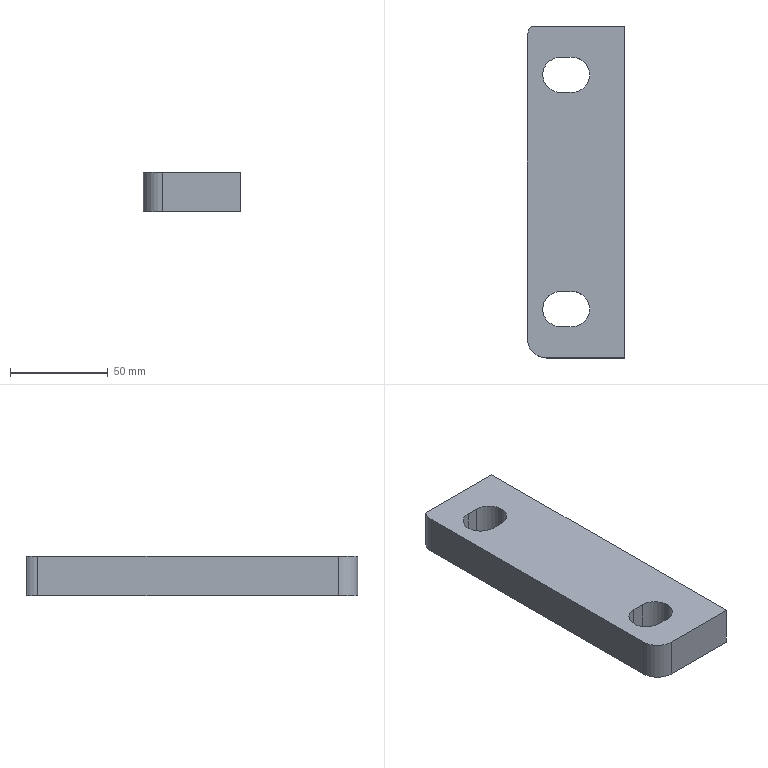Part | SolidWorks | features BaseBody 1 | 1 solid | 18 faces | box 50 x 170 x 20 mm | volume 154996 mm3 | plane 10 | cylinder 8 | commonest cylinder face diameters 18 x6 20 x2
STEP:
#1=CARTESIAN_POINT('',(-40.5,-55.,-12.5));
#2=VERTEX_POINT('',#1);
#3=CARTESIAN_POINT('',(-49.5,-46.,-12.5));
#4=VERTEX_POINT('',#3);
#5=CARTESIAN_POINT('',(-49.5,-55.,-12.5));
#6=DIRECTION('',(0.,0.,1.));
#7=DIRECTION('',(1.,0.,0.));
#8=AXIS2_PLACEMENT_3D('',#5,#6,#7);
#9=CIRCLE('',#8,9.);
#10=EDGE_CURVE('',#2,#4,#9,.T.);
#11=ORIENTED_EDGE('',*,*,#10,.F.);
#12=CARTESIAN_POINT('',(-40.5,-55.,7.5));
#13=VERTEX_POINT('',#12);
#14=CARTESIAN_POINT('',(-40.5,-55.,-12.5));
#15=DIRECTION('',(0.,0.,1.));
#16=VECTOR('',#15,1000.);
#17=LINE('',#14,#16);
#18=EDGE_CURVE('',#2,#13,#17,.T.);
#19=ORIENTED_EDGE('',*,*,#18,.T.);
#20=CARTESIAN_POINT('',(-49.5,-46.,7.5));
#21=VERTEX_POINT('',#20);
#22=CARTESIAN_POINT('',(-49.5,-55.,7.5));
#23=DIRECTION('',(0.,0.,1.));
#24=DIRECTION('',(1.,0.,0.));
#25=AXIS2_PLACEMENT_3D('',#22,#23,#24);
#26=CIRCLE('',#25,9.);
#27=EDGE_CURVE('',#13,#21,#26,.T.);
#28=ORIENTED_EDGE('',*,*,#27,.T.);
#29=CARTESIAN_POINT('',(-49.5,-46.,-12.5));
#30=DIRECTION('',(0.,0.,1.));
#31=VECTOR('',#30,1000.);
#32=LINE('',#29,#31);
#33=EDGE_CURVE('',#4,#21,#32,.T.);
#34=ORIENTED_EDGE('',*,*,#33,.F.);
#35=EDGE_LOOP('',(#11,#19,#28,#34));
#36=FACE_OUTER_BOUND('',#35,.T.);
#37=CARTESIAN_POINT('',(-49.5,-55.,-12.5));
#38=DIRECTION('',(0.,0.,1.));
#39=DIRECTION('',(1.,0.,0.));
#40=AXIS2_PLACEMENT_3D('',#37,#38,#39);
#41=CYLINDRICAL_SURFACE('',#40,9.);
#42=ADVANCED_FACE('',(#36),#41,.F.);
#43=CARTESIAN_POINT('',(-40.5,65.,-12.5));
#44=VERTEX_POINT('',#43);
#45=CARTESIAN_POINT('',(-49.5,74.,-12.5));
#46=VERTEX_POINT('',#45);
#47=CARTESIAN_POINT('',(-49.5,65.,-12.5));
#48=DIRECTION('',(0.,0.,1.));
#49=DIRECTION('',(1.,0.,0.));
#50=AXIS2_PLACEMENT_3D('',#47,#48,#49);
#51=CIRCLE('',#50,9.);
#52=EDGE_CURVE('',#44,#46,#51,.T.);
#53=ORIENTED_EDGE('',*,*,#52,.F.);
#54=CARTESIAN_POINT('',(-40.5,65.,7.5));
#55=VERTEX_POINT('',#54);
#56=CARTESIAN_POINT('',(-40.5,65.,-12.5));
#57=DIRECTION('',(0.,0.,1.));
#58=VECTOR('',#57,1000.);
#59=LINE('',#56,#58);
#60=EDGE_CURVE('',#44,#55,#59,.T.);
#61=ORIENTED_EDGE('',*,*,#60,.T.);
#62=CARTESIAN_POINT('',(-49.5,74.,7.5));
#63=VERTEX_POINT('',#62);
#64=CARTESIAN_POINT('',(-49.5,65.,7.5));
#65=DIRECTION('',(0.,0.,1.));
#66=DIRECTION('',(1.,0.,0.));
#67=AXIS2_PLACEMENT_3D('',#64,#65,#66);
#68=CIRCLE('',#67,9.);
#69=EDGE_CURVE('',#55,#63,#68,.T.);
#70=ORIENTED_EDGE('',*,*,#69,.T.);
#71=CARTESIAN_POINT('',(-49.5,74.,-12.5));
#72=DIRECTION('',(0.,0.,1.));
#73=VECTOR('',#72,1000.);
#74=LINE('',#71,#73);
#75=EDGE_CURVE('',#46,#63,#74,.T.);
#76=ORIENTED_EDGE('',*,*,#75,.F.);
#77=EDGE_LOOP('',(#53,#61,#70,#76));
#78=FACE_OUTER_BOUND('',#77,.T.);
#79=CARTESIAN_POINT('',(-49.5,65.,-12.5));
#80=DIRECTION('',(0.,0.,1.));
#81=DIRECTION('',(1.,0.,0.));
#82=AXIS2_PLACEMENT_3D('',#79,#80,#81);
#83=CYLINDRICAL_SURFACE('',#82,9.);
#84=ADVANCED_FACE('',(#78),#83,.F.);
#85=CARTESIAN_POINT('',(-22.5,-80.,7.5));
#86=VERTEX_POINT('',#85);
#87=CARTESIAN_POINT('',(-22.5,90.,7.5));
#88=VERTEX_POINT('',#87);
#89=CARTESIAN_POINT('',(-22.5,94.,7.5));
#90=DIRECTION('',(0.,1.,0.));
#91=VECTOR('',#90,1000.);
#92=LINE('',#89,#91);
#93=EDGE_CURVE('',#86,#88,#92,.T.);
#94=ORIENTED_EDGE('',*,*,#93,.F.);
#95=CARTESIAN_POINT('',(-22.5,-80.,-12.5));
#96=VERTEX_POINT('',#95);
#97=CARTESIAN_POINT('',(-22.5,-80.,12.5));
#98=DIRECTION('',(0.,0.,-1.));
#99=VECTOR('',#98,1000.);
#100=LINE('',#97,#99);
#101=EDGE_CURVE('',#86,#96,#100,.T.);
#102=ORIENTED_EDGE('',*,*,#101,.T.);
#103=CARTESIAN_POINT('',(-22.5,90.,-12.5));
#104=VERTEX_POINT('',#103);
#105=CARTESIAN_POINT('',(-22.5,94.,-12.5));
#106=DIRECTION('',(0.,1.,0.));
#107=VECTOR('',#106,1000.);
#108=LINE('',#105,#107);
#109=EDGE_CURVE('',#96,#104,#108,.T.);
#110=ORIENTED_EDGE('',*,*,#109,.T.);
#111=CARTESIAN_POINT('',(-22.5,90.,12.5));
#112=DIRECTION('',(0.,0.,-1.));
#113=VECTOR('',#112,1000.);
#114=LINE('',#111,#113);
#115=EDGE_CURVE('',#88,#104,#114,.T.);
#116=ORIENTED_EDGE('',*,*,#115,.F.);
#117=EDGE_LOOP('',(#94,#102,#110,#116));
#118=FACE_OUTER_BOUND('',#117,.T.);
#119=CARTESIAN_POINT('',(-22.5,94.,12.5));
#120=DIRECTION('',(-1.,0.,0.));
#121=DIRECTION('',(0.,-1.,0.));
#122=AXIS2_PLACEMENT_3D('',#119,#120,#121);
#123=PLANE('',#122);
#124=ADVANCED_FACE('',(#118),#123,.F.);
#125=CARTESIAN_POINT('',(-70.5,90.,7.5));
#126=VERTEX_POINT('',#125);
#127=CARTESIAN_POINT('',(-72.5,84.,7.5));
#128=VERTEX_POINT('',#127);
#129=CARTESIAN_POINT('',(-62.5,84.,7.5));
#130=DIRECTION('',(0.,0.,1.));
#131=DIRECTION('',(0.,-1.,0.));
#132=AXIS2_PLACEMENT_3D('',#129,#130,#131);
#133=CIRCLE('',#132,10.);
#134=EDGE_CURVE('',#126,#128,#133,.T.);
#135=ORIENTED_EDGE('',*,*,#134,.F.);
#136=CARTESIAN_POINT('',(-70.5,90.,-12.5));
#137=VERTEX_POINT('',#136);
#138=CARTESIAN_POINT('',(-70.5,90.,12.5));
#139=DIRECTION('',(0.,0.,1.));
#140=VECTOR('',#139,1000.);
#141=LINE('',#138,#140);
#142=EDGE_CURVE('',#137,#126,#141,.T.);
#143=ORIENTED_EDGE('',*,*,#142,.F.);
#144=CARTESIAN_POINT('',(-72.5,84.,-12.5));
#145=VERTEX_POINT('',#144);
#146=CARTESIAN_POINT('',(-62.5,84.,-12.5));
#147=DIRECTION('',(0.,0.,1.));
#148=DIRECTION('',(1.,0.,0.));
#149=AXIS2_PLACEMENT_3D('',#146,#147,#148);
#150=CIRCLE('',#149,10.);
#151=EDGE_CURVE('',#137,#145,#150,.T.);
#152=ORIENTED_EDGE('',*,*,#151,.T.);
#153=CARTESIAN_POINT('',(-72.5,84.,12.5));
#154=DIRECTION('',(0.,0.,-1.));
#155=VECTOR('',#154,1000.);
#156=LINE('',#153,#155);
#157=EDGE_CURVE('',#128,#145,#156,.T.);
#158=ORIENTED_EDGE('',*,*,#157,.F.);
#159=EDGE_LOOP('',(#135,#143,#152,#158));
#160=FACE_OUTER_BOUND('',#159,.T.);
#161=CARTESIAN_POINT('',(-62.5,84.,12.5));
#162=DIRECTION('',(0.,0.,-1.));
#163=DIRECTION('',(-1.,0.,0.));
#164=AXIS2_PLACEMENT_3D('',#161,#162,#163);
#165=CYLINDRICAL_SURFACE('',#164,10.);
#166=ADVANCED_FACE('',(#160),#165,.T.);
#167=CARTESIAN_POINT('',(-72.5,-70.,7.5));
#168=VERTEX_POINT('',#167);
#169=CARTESIAN_POINT('',(-72.5,84.,7.5));
#170=DIRECTION('',(0.,-1.,0.));
#171=VECTOR('',#170,1000.);
#172=LINE('',#169,#171);
#173=EDGE_CURVE('',#128,#168,#172,.T.);
#174=ORIENTED_EDGE('',*,*,#173,.F.);
#175=ORIENTED_EDGE('',*,*,#157,.T.);
#176=CARTESIAN_POINT('',(-72.5,-70.,-12.5));
#177=VERTEX_POINT('',#176);
#178=CARTESIAN_POINT('',(-72.5,84.,-12.5));
#179=DIRECTION('',(0.,-1.,0.));
#180=VECTOR('',#179,1000.);
#181=LINE('',#178,#180);
#182=EDGE_CURVE('',#145,#177,#181,.T.);
#183=ORIENTED_EDGE('',*,*,#182,.T.);
#184=CARTESIAN_POINT('',(-72.5,-70.,12.5));
#185=DIRECTION('',(0.,0.,-1.));
#186=VECTOR('',#185,1000.);
#187=LINE('',#184,#186);
#188=EDGE_CURVE('',#168,#177,#187,.T.);
#189=ORIENTED_EDGE('',*,*,#188,.F.);
#190=EDGE_LOOP('',(#174,#175,#183,#189));
#191=FACE_OUTER_BOUND('',#190,.T.);
#192=CARTESIAN_POINT('',(-72.5,84.,12.5));
#193=DIRECTION('',(1.,0.,0.));
#194=DIRECTION('',(0.,1.,0.));
#195=AXIS2_PLACEMENT_3D('',#192,#193,#194);
#196=PLANE('',#195);
#197=ADVANCED_FACE('',(#191),#196,.F.);
#198=CARTESIAN_POINT('',(-62.5,-80.,7.5));
#199=VERTEX_POINT('',#198);
#200=CARTESIAN_POINT('',(-62.5,-70.,7.5));
#201=DIRECTION('',(0.,0.,1.));
#202=DIRECTION('',(0.,-1.,0.));
#203=AXIS2_PLACEMENT_3D('',#200,#201,#202);
#204=CIRCLE('',#203,10.);
#205=EDGE_CURVE('',#168,#199,#204,.T.);
#206=ORIENTED_EDGE('',*,*,#205,.F.);
#207=ORIENTED_EDGE('',*,*,#188,.T.);
#208=CARTESIAN_POINT('',(-62.5,-80.,-12.5));
#209=VERTEX_POINT('',#208);
#210=CARTESIAN_POINT('',(-62.5,-70.,-12.5));
#211=DIRECTION('',(0.,0.,1.));
#212=DIRECTION('',(1.,0.,0.));
#213=AXIS2_PLACEMENT_3D('',#210,#211,#212);
#214=CIRCLE('',#213,10.);
#215=EDGE_CURVE('',#177,#209,#214,.T.);
#216=ORIENTED_EDGE('',*,*,#215,.T.);
#217=CARTESIAN_POINT('',(-62.5,-80.,12.5));
#218=DIRECTION('',(0.,0.,-1.));
#219=VECTOR('',#218,1000.);
#220=LINE('',#217,#219);
#221=EDGE_CURVE('',#199,#209,#220,.T.);
#222=ORIENTED_EDGE('',*,*,#221,.F.);
#223=EDGE_LOOP('',(#206,#207,#216,#222));
#224=FACE_OUTER_BOUND('',#223,.T.);
#225=CARTESIAN_POINT('',(-62.5,-70.,12.5));
#226=DIRECTION('',(0.,0.,-1.));
#227=DIRECTION('',(-1.,0.,0.));
#228=AXIS2_PLACEMENT_3D('',#225,#226,#227);
#229=CYLINDRICAL_SURFACE('',#228,10.);
#230=ADVANCED_FACE('',(#224),#229,.T.);
#231=CARTESIAN_POINT('',(-1372.5,-80.,7.5));
#232=DIRECTION('',(1.,0.,0.));
#233=VECTOR('',#232,1000.);
#234=LINE('',#231,#233);
#235=EDGE_CURVE('',#199,#86,#234,.T.);
#236=ORIENTED_EDGE('',*,*,#235,.F.);
#237=ORIENTED_EDGE('',*,*,#221,.T.);
#238=CARTESIAN_POINT('',(-62.5,-80.,-12.5));
#239=DIRECTION('',(1.,0.,0.));
#240=VECTOR('',#239,1000.);
#241=LINE('',#238,#240);
#242=EDGE_CURVE('',#209,#96,#241,.T.);
#243=ORIENTED_EDGE('',*,*,#242,.T.);
#244=ORIENTED_EDGE('',*,*,#101,.F.);
#245=EDGE_LOOP('',(#236,#237,#243,#244));
#246=FACE_OUTER_BOUND('',#245,.T.);
#247=CARTESIAN_POINT('',(-62.5,-80.,12.5));
#248=DIRECTION('',(0.,1.,0.));
#249=DIRECTION('',(0.,0.,1.));
#250=AXIS2_PLACEMENT_3D('',#247,#248,#249);
#251=PLANE('',#250);
#252=ADVANCED_FACE('',(#246),#251,.F.);
#253=ORIENTED_EDGE('',*,*,#142,.T.);
#254=CARTESIAN_POINT('',(-657.5,90.,7.5));
#255=DIRECTION('',(1.,0.,0.));
#256=VECTOR('',#255,1000.);
#257=LINE('',#254,#256);
#258=EDGE_CURVE('',#126,#88,#257,.T.);
#259=ORIENTED_EDGE('',*,*,#258,.T.);
#260=ORIENTED_EDGE('',*,*,#115,.T.);
#261=CARTESIAN_POINT('',(-62.5,90.,-12.5));
#262=DIRECTION('',(-1.,0.,0.));
#263=VECTOR('',#262,1000.);
#264=LINE('',#261,#263);
#265=EDGE_CURVE('',#104,#137,#264,.T.);
#266=ORIENTED_EDGE('',*,*,#265,.T.);
#267=EDGE_LOOP('',(#253,#259,#260,#266));
#268=FACE_OUTER_BOUND('',#267,.T.);
#269=CARTESIAN_POINT('',(-657.5,90.,-755.));
#270=DIRECTION('',(0.,1.,0.));
#271=DIRECTION('',(0.,0.,1.));
#272=AXIS2_PLACEMENT_3D('',#269,#270,#271);
#273=PLANE('',#272);
#274=ADVANCED_FACE('',(#268),#273,.T.);
#275=CARTESIAN_POINT('',(-55.5,-46.,-12.5));
#276=VERTEX_POINT('',#275);
#277=CARTESIAN_POINT('',(-55.5,-46.,-12.5));
#278=DIRECTION('',(-1.,0.,0.));
#279=VECTOR('',#278,1000.);
#280=LINE('',#277,#279);
#281=EDGE_CURVE('',#4,#276,#280,.T.);
#282=ORIENTED_EDGE('',*,*,#281,.T.);
#283=CARTESIAN_POINT('',(-55.5,-64.,-12.5));
#284=VERTEX_POINT('',#283);
#285=CARTESIAN_POINT('',(-55.5,-55.,-12.5));
#286=DIRECTION('',(0.,0.,1.));
#287=DIRECTION('',(1.,0.,0.));
#288=AXIS2_PLACEMENT_3D('',#285,#286,#287);
#289=CIRCLE('',#288,9.);
#290=EDGE_CURVE('',#276,#284,#289,.T.);
#291=ORIENTED_EDGE('',*,*,#290,.T.);
#292=CARTESIAN_POINT('',(-49.5,-64.,-12.5));
#293=VERTEX_POINT('',#292);
#294=CARTESIAN_POINT('',(-55.5,-64.,-12.5));
#295=DIRECTION('',(1.,0.,0.));
#296=VECTOR('',#295,1000.);
#297=LINE('',#294,#296);
#298=EDGE_CURVE('',#284,#293,#297,.T.);
#299=ORIENTED_EDGE('',*,*,#298,.T.);
#300=CARTESIAN_POINT('',(-49.5,-55.,-12.5));
#301=DIRECTION('',(0.,0.,1.));
#302=DIRECTION('',(1.,0.,0.));
#303=AXIS2_PLACEMENT_3D('',#300,#301,#302);
#304=CIRCLE('',#303,9.);
#305=EDGE_CURVE('',#293,#2,#304,.T.);
#306=ORIENTED_EDGE('',*,*,#305,.T.);
#307=ORIENTED_EDGE('',*,*,#10,.T.);
#308=EDGE_LOOP('',(#282,#291,#299,#306,#307));
#309=FACE_BOUND('',#308,.T.);
#310=CARTESIAN_POINT('',(-55.5,74.,-12.5));
#311=VERTEX_POINT('',#310);
#312=CARTESIAN_POINT('',(-55.5,74.,-12.5));
#313=DIRECTION('',(-1.,0.,0.));
#314=VECTOR('',#313,1000.);
#315=LINE('',#312,#314);
#316=EDGE_CURVE('',#46,#311,#315,.T.);
#317=ORIENTED_EDGE('',*,*,#316,.T.);
#318=CARTESIAN_POINT('',(-55.5,56.,-12.5));
#319=VERTEX_POINT('',#318);
#320=CARTESIAN_POINT('',(-55.5,65.,-12.5));
#321=DIRECTION('',(0.,0.,1.));
#322=DIRECTION('',(1.,0.,0.));
#323=AXIS2_PLACEMENT_3D('',#320,#321,#322);
#324=CIRCLE('',#323,9.);
#325=EDGE_CURVE('',#311,#319,#324,.T.);
#326=ORIENTED_EDGE('',*,*,#325,.T.);
#327=CARTESIAN_POINT('',(-49.5,56.,-12.5));
#328=VERTEX_POINT('',#327);
#329=CARTESIAN_POINT('',(-55.5,56.,-12.5));
#330=DIRECTION('',(1.,0.,0.));
#331=VECTOR('',#330,1000.);
#332=LINE('',#329,#331);
#333=EDGE_CURVE('',#319,#328,#332,.T.);
#334=ORIENTED_EDGE('',*,*,#333,.T.);
#335=CARTESIAN_POINT('',(-49.5,65.,-12.5));
#336=DIRECTION('',(0.,0.,1.));
#337=DIRECTION('',(1.,0.,0.));
#338=AXIS2_PLACEMENT_3D('',#335,#336,#337);
#339=CIRCLE('',#338,9.);
#340=EDGE_CURVE('',#328,#44,#339,.T.);
#341=ORIENTED_EDGE('',*,*,#340,.T.);
#342=ORIENTED_EDGE('',*,*,#52,.T.);
#343=EDGE_LOOP('',(#317,#326,#334,#341,#342));
#344=FACE_BOUND('',#343,.T.);
#345=ORIENTED_EDGE('',*,*,#265,.F.);
#346=ORIENTED_EDGE('',*,*,#109,.F.);
#347=ORIENTED_EDGE('',*,*,#242,.F.);
#348=ORIENTED_EDGE('',*,*,#215,.F.);
#349=ORIENTED_EDGE('',*,*,#182,.F.);
#350=ORIENTED_EDGE('',*,*,#151,.F.);
#351=EDGE_LOOP('',(#345,#346,#347,#348,#349,#350));
#352=FACE_OUTER_BOUND('',#351,.T.);
#353=CARTESIAN_POINT('',(-62.5,-70.,-12.5));
#354=DIRECTION('',(0.,0.,1.));
#355=DIRECTION('',(1.,0.,0.));
#356=AXIS2_PLACEMENT_3D('',#353,#354,#355);
#357=PLANE('',#356);
#358=ADVANCED_FACE('',(#309,#344,#352),#357,.F.);
#359=CARTESIAN_POINT('',(-55.5,-46.,7.5));
#360=VERTEX_POINT('',#359);
#361=CARTESIAN_POINT('',(-55.5,-64.,7.5));
#362=VERTEX_POINT('',#361);
#363=CARTESIAN_POINT('',(-55.5,-55.,7.5));
#364=DIRECTION('',(0.,0.,1.));
#365=DIRECTION('',(1.,0.,0.));
#366=AXIS2_PLACEMENT_3D('',#363,#364,#365);
#367=CIRCLE('',#366,9.);
#368=EDGE_CURVE('',#360,#362,#367,.T.);
#369=ORIENTED_EDGE('',*,*,#368,.F.);
#370=CARTESIAN_POINT('',(-55.5,-46.,7.5));
#371=DIRECTION('',(-1.,0.,0.));
#372=VECTOR('',#371,1000.);
#373=LINE('',#370,#372);
#374=EDGE_CURVE('',#21,#360,#373,.T.);
#375=ORIENTED_EDGE('',*,*,#374,.F.);
#376=ORIENTED_EDGE('',*,*,#27,.F.);
#377=CARTESIAN_POINT('',(-49.5,-64.,7.5));
#378=VERTEX_POINT('',#377);
#379=CARTESIAN_POINT('',(-49.5,-55.,7.5));
#380=DIRECTION('',(0.,0.,1.));
#381=DIRECTION('',(1.,0.,0.));
#382=AXIS2_PLACEMENT_3D('',#379,#380,#381);
#383=CIRCLE('',#382,9.);
#384=EDGE_CURVE('',#378,#13,#383,.T.);
#385=ORIENTED_EDGE('',*,*,#384,.F.);
#386=CARTESIAN_POINT('',(-55.5,-64.,7.5));
#387=DIRECTION('',(1.,0.,0.));
#388=VECTOR('',#387,1000.);
#389=LINE('',#386,#388);
#390=EDGE_CURVE('',#362,#378,#389,.T.);
#391=ORIENTED_EDGE('',*,*,#390,.F.);
#392=EDGE_LOOP('',(#369,#375,#376,#385,#391));
#393=FACE_BOUND('',#392,.T.);
#394=CARTESIAN_POINT('',(-55.5,74.,7.5));
#395=VERTEX_POINT('',#394);
#396=CARTESIAN_POINT('',(-55.5,56.,7.5));
#397=VERTEX_POINT('',#396);
#398=CARTESIAN_POINT('',(-55.5,65.,7.5));
#399=DIRECTION('',(0.,0.,1.));
#400=DIRECTION('',(1.,0.,0.));
#401=AXIS2_PLACEMENT_3D('',#398,#399,#400);
#402=CIRCLE('',#401,9.);
#403=EDGE_CURVE('',#395,#397,#402,.T.);
#404=ORIENTED_EDGE('',*,*,#403,.F.);
#405=CARTESIAN_POINT('',(-55.5,74.,7.5));
#406=DIRECTION('',(-1.,0.,0.));
#407=VECTOR('',#406,1000.);
#408=LINE('',#405,#407);
#409=EDGE_CURVE('',#63,#395,#408,.T.);
#410=ORIENTED_EDGE('',*,*,#409,.F.);
#411=ORIENTED_EDGE('',*,*,#69,.F.);
#412=CARTESIAN_POINT('',(-49.5,56.,7.5));
#413=VERTEX_POINT('',#412);
#414=CARTESIAN_POINT('',(-49.5,65.,7.5));
#415=DIRECTION('',(0.,0.,1.));
#416=DIRECTION('',(1.,0.,0.));
#417=AXIS2_PLACEMENT_3D('',#414,#415,#416);
#418=CIRCLE('',#417,9.);
#419=EDGE_CURVE('',#413,#55,#418,.T.);
#420=ORIENTED_EDGE('',*,*,#419,.F.);
#421=CARTESIAN_POINT('',(-55.5,56.,7.5));
#422=DIRECTION('',(1.,0.,0.));
#423=VECTOR('',#422,1000.);
#424=LINE('',#421,#423);
#425=EDGE_CURVE('',#397,#413,#424,.T.);
#426=ORIENTED_EDGE('',*,*,#425,.F.);
#427=EDGE_LOOP('',(#404,#410,#411,#420,#426));
#428=FACE_BOUND('',#427,.T.);
#429=ORIENTED_EDGE('',*,*,#93,.T.);
#430=ORIENTED_EDGE('',*,*,#258,.F.);
#431=ORIENTED_EDGE('',*,*,#134,.T.);
#432=ORIENTED_EDGE('',*,*,#173,.T.);
#433=ORIENTED_EDGE('',*,*,#205,.T.);
#434=ORIENTED_EDGE('',*,*,#235,.T.);
#435=EDGE_LOOP('',(#429,#430,#431,#432,#433,#434));
#436=FACE_OUTER_BOUND('',#435,.T.);
#437=CARTESIAN_POINT('',(-657.5,0.,7.5));
#438=DIRECTION('',(0.,0.,1.));
#439=DIRECTION('',(1.,0.,0.));
#440=AXIS2_PLACEMENT_3D('',#437,#438,#439);
#441=PLANE('',#440);
#442=ADVANCED_FACE('',(#393,#428,#436),#441,.T.);
#443=ORIENTED_EDGE('',*,*,#403,.T.);
#444=CARTESIAN_POINT('',(-55.5,56.,-12.5));
#445=DIRECTION('',(0.,0.,1.));
#446=VECTOR('',#445,1000.);
#447=LINE('',#444,#446);
#448=EDGE_CURVE('',#319,#397,#447,.T.);
#449=ORIENTED_EDGE('',*,*,#448,.F.);
#450=ORIENTED_EDGE('',*,*,#325,.F.);
#451=CARTESIAN_POINT('',(-55.5,74.,-12.5));
#452=DIRECTION('',(0.,0.,1.));
#453=VECTOR('',#452,1000.);
#454=LINE('',#451,#453);
#455=EDGE_CURVE('',#311,#395,#454,.T.);
#456=ORIENTED_EDGE('',*,*,#455,.T.);
#457=EDGE_LOOP('',(#443,#449,#450,#456));
#458=FACE_OUTER_BOUND('',#457,.T.);
#459=CARTESIAN_POINT('',(-55.5,65.,-12.5));
#460=DIRECTION('',(0.,0.,1.));
#461=DIRECTION('',(1.,0.,0.));
#462=AXIS2_PLACEMENT_3D('',#459,#460,#461);
#463=CYLINDRICAL_SURFACE('',#462,9.);
#464=ADVANCED_FACE('',(#458),#463,.F.);
#465=ORIENTED_EDGE('',*,*,#409,.T.);
#466=ORIENTED_EDGE('',*,*,#455,.F.);
#467=ORIENTED_EDGE('',*,*,#316,.F.);
#468=ORIENTED_EDGE('',*,*,#75,.T.);
#469=EDGE_LOOP('',(#465,#466,#467,#468));
#470=FACE_OUTER_BOUND('',#469,.T.);
#471=CARTESIAN_POINT('',(-55.5,74.,-12.5));
#472=DIRECTION('',(0.,1.,0.));
#473=DIRECTION('',(0.,0.,1.));
#474=AXIS2_PLACEMENT_3D('',#471,#472,#473);
#475=PLANE('',#474);
#476=ADVANCED_FACE('',(#470),#475,.F.);
#477=ORIENTED_EDGE('',*,*,#60,.F.);
#478=ORIENTED_EDGE('',*,*,#340,.F.);
#479=CARTESIAN_POINT('',(-49.5,56.,-12.5));
#480=DIRECTION('',(0.,0.,1.));
#481=VECTOR('',#480,1000.);
#482=LINE('',#479,#481);
#483=EDGE_CURVE('',#328,#413,#482,.T.);
#484=ORIENTED_EDGE('',*,*,#483,.T.);
#485=ORIENTED_EDGE('',*,*,#419,.T.);
#486=EDGE_LOOP('',(#477,#478,#484,#485));
#487=FACE_OUTER_BOUND('',#486,.T.);
#488=CARTESIAN_POINT('',(-49.5,65.,-12.5));
#489=DIRECTION('',(0.,0.,1.));
#490=DIRECTION('',(1.,0.,0.));
#491=AXIS2_PLACEMENT_3D('',#488,#489,#490);
#492=CYLINDRICAL_SURFACE('',#491,9.);
#493=ADVANCED_FACE('',(#487),#492,.F.);
#494=ORIENTED_EDGE('',*,*,#425,.T.);
#495=ORIENTED_EDGE('',*,*,#483,.F.);
#496=ORIENTED_EDGE('',*,*,#333,.F.);
#497=ORIENTED_EDGE('',*,*,#448,.T.);
#498=EDGE_LOOP('',(#494,#495,#496,#497));
#499=FACE_OUTER_BOUND('',#498,.T.);
#500=CARTESIAN_POINT('',(-55.5,56.,-12.5));
#501=DIRECTION('',(0.,-1.,0.));
#502=DIRECTION('',(0.,0.,-1.));
#503=AXIS2_PLACEMENT_3D('',#500,#501,#502);
#504=PLANE('',#503);
#505=ADVANCED_FACE('',(#499),#504,.F.);
#506=ORIENTED_EDGE('',*,*,#368,.T.);
#507=CARTESIAN_POINT('',(-55.5,-64.,-12.5));
#508=DIRECTION('',(0.,0.,1.));
#509=VECTOR('',#508,1000.);
#510=LINE('',#507,#509);
#511=EDGE_CURVE('',#284,#362,#510,.T.);
#512=ORIENTED_EDGE('',*,*,#511,.F.);
#513=ORIENTED_EDGE('',*,*,#290,.F.);
#514=CARTESIAN_POINT('',(-55.5,-46.,-12.5));
#515=DIRECTION('',(0.,0.,1.));
#516=VECTOR('',#515,1000.);
#517=LINE('',#514,#516);
#518=EDGE_CURVE('',#276,#360,#517,.T.);
#519=ORIENTED_EDGE('',*,*,#518,.T.);
#520=EDGE_LOOP('',(#506,#512,#513,#519));
#521=FACE_OUTER_BOUND('',#520,.T.);
#522=CARTESIAN_POINT('',(-55.5,-55.,-12.5));
#523=DIRECTION('',(0.,0.,1.));
#524=DIRECTION('',(1.,0.,0.));
#525=AXIS2_PLACEMENT_3D('',#522,#523,#524);
#526=CYLINDRICAL_SURFACE('',#525,9.);
#527=ADVANCED_FACE('',(#521),#526,.F.);
#528=ORIENTED_EDGE('',*,*,#374,.T.);
#529=ORIENTED_EDGE('',*,*,#518,.F.);
#530=ORIENTED_EDGE('',*,*,#281,.F.);
#531=ORIENTED_EDGE('',*,*,#33,.T.);
#532=EDGE_LOOP('',(#528,#529,#530,#531));
#533=FACE_OUTER_BOUND('',#532,.T.);
#534=CARTESIAN_POINT('',(-55.5,-46.,-12.5));
#535=DIRECTION('',(0.,1.,0.));
#536=DIRECTION('',(0.,0.,1.));
#537=AXIS2_PLACEMENT_3D('',#534,#535,#536);
#538=PLANE('',#537);
#539=ADVANCED_FACE('',(#533),#538,.F.);
#540=ORIENTED_EDGE('',*,*,#18,.F.);
#541=ORIENTED_EDGE('',*,*,#305,.F.);
#542=CARTESIAN_POINT('',(-49.5,-64.,-12.5));
#543=DIRECTION('',(0.,0.,1.));
#544=VECTOR('',#543,1000.);
#545=LINE('',#542,#544);
#546=EDGE_CURVE('',#293,#378,#545,.T.);
#547=ORIENTED_EDGE('',*,*,#546,.T.);
#548=ORIENTED_EDGE('',*,*,#384,.T.);
#549=EDGE_LOOP('',(#540,#541,#547,#548));
#550=FACE_OUTER_BOUND('',#549,.T.);
#551=CARTESIAN_POINT('',(-49.5,-55.,-12.5));
#552=DIRECTION('',(0.,0.,1.));
#553=DIRECTION('',(1.,0.,0.));
#554=AXIS2_PLACEMENT_3D('',#551,#552,#553);
#555=CYLINDRICAL_SURFACE('',#554,9.);
#556=ADVANCED_FACE('',(#550),#555,.F.);
#557=ORIENTED_EDGE('',*,*,#390,.T.);
#558=ORIENTED_EDGE('',*,*,#546,.F.);
#559=ORIENTED_EDGE('',*,*,#298,.F.);
#560=ORIENTED_EDGE('',*,*,#511,.T.);
#561=EDGE_LOOP('',(#557,#558,#559,#560));
#562=FACE_OUTER_BOUND('',#561,.T.);
#563=CARTESIAN_POINT('',(-55.5,-64.,-12.5));
#564=DIRECTION('',(0.,-1.,0.));
#565=DIRECTION('',(0.,0.,-1.));
#566=AXIS2_PLACEMENT_3D('',#563,#564,#565);
#567=PLANE('',#566);
#568=ADVANCED_FACE('',(#562),#567,.F.);
#569=CLOSED_SHELL('',(#42,#84,#124,#166,#197,#230,#252,#274,#358,#442,#464,#476,#493,#505,#527,#539,#556,#568));
#570=MANIFOLD_SOLID_BREP('',#569);
#571=CARTESIAN_POINT('',(0.,0.,0.));
#572=DIRECTION('',(0.,0.,1.));
#573=DIRECTION('',(1.,0.,0.));
#574=AXIS2_PLACEMENT_3D('',#571,#572,#573);
#575=(LENGTH_UNIT()NAMED_UNIT(*)SI_UNIT(.MILLI.,.METRE.));
#576=UNCERTAINTY_MEASURE_WITH_UNIT(LENGTH_MEASURE(0.00001),#575,'','');
#577=(NAMED_UNIT(*)PLANE_ANGLE_UNIT()SI_UNIT($,.RADIAN.));
#578=(NAMED_UNIT(*)SI_UNIT($,.STERADIAN.)SOLID_ANGLE_UNIT());
#579=(GEOMETRIC_REPRESENTATION_CONTEXT(3)GLOBAL_UNCERTAINTY_ASSIGNED_CONTEXT((#576))GLOBAL_UNIT_ASSIGNED_CONTEXT((#575,#577,#578))REPRESENTATION_CONTEXT('',''));
#580=ADVANCED_BREP_SHAPE_REPRESENTATION('',(#570,#574),#579);